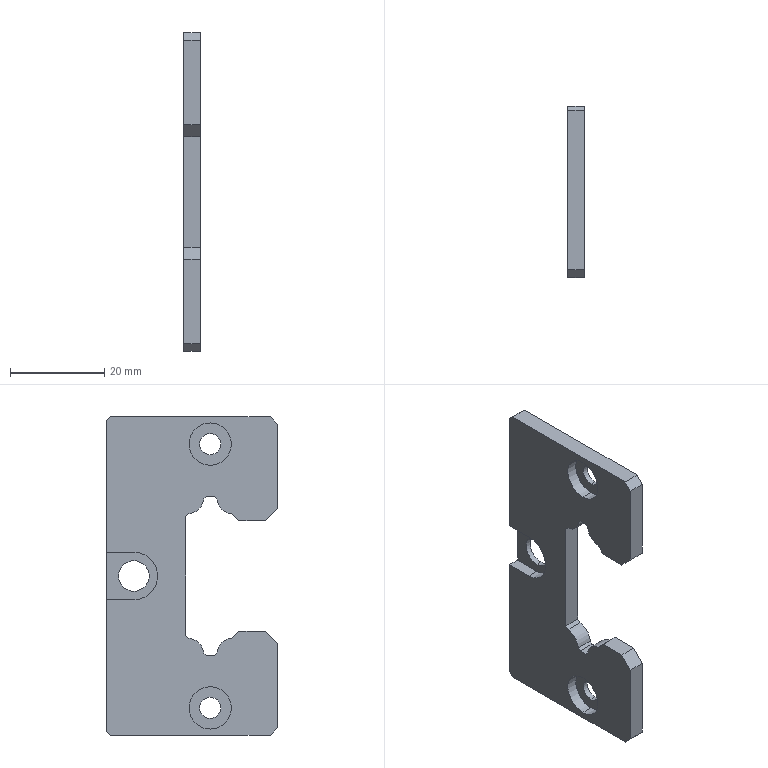Part | STEP file | _MSA35ES | 1 solid | 46 faces | box 3.6 x 36.3 x 67.6 mm | volume 6318 mm3 | plane 31 | cylinder 15 | commonest cylinder face diameters 4.5 x4 7 x4 9 x4 6.5 x2 10.1 x1
STEP:
#1=CARTESIAN_POINT('',(2.4,23.85,30.25));
#2=VERTEX_POINT('',#1);
#3=CARTESIAN_POINT('',(2.4,23.85,25.75));
#4=VERTEX_POINT('',#3);
#5=CARTESIAN_POINT('',(2.4,23.85,28.));
#6=DIRECTION('',(1.,0.,0.));
#7=DIRECTION('',(0.,0.,-1.));
#8=AXIS2_PLACEMENT_3D('',#5,#6,#7);
#9=CIRCLE('',#8,2.25);
#10=EDGE_CURVE('',#2,#4,#9,.T.);
#11=ORIENTED_EDGE('',*,*,#10,.F.);
#12=CARTESIAN_POINT('',(3.6,23.85,30.25));
#13=VERTEX_POINT('',#12);
#14=CARTESIAN_POINT('',(3.6,23.85,30.25));
#15=DIRECTION('',(1.,0.,0.));
#16=VECTOR('',#15,1000.);
#17=LINE('',#14,#16);
#18=EDGE_CURVE('',#2,#13,#17,.T.);
#19=ORIENTED_EDGE('',*,*,#18,.T.);
#20=CARTESIAN_POINT('',(3.6,23.85,25.75));
#21=VERTEX_POINT('',#20);
#22=CARTESIAN_POINT('',(3.6,23.85,28.));
#23=DIRECTION('',(-1.,0.,0.));
#24=DIRECTION('',(0.,0.,-1.));
#25=AXIS2_PLACEMENT_3D('',#22,#23,#24);
#26=CIRCLE('',#25,2.25);
#27=EDGE_CURVE('',#21,#13,#26,.T.);
#28=ORIENTED_EDGE('',*,*,#27,.F.);
#29=CARTESIAN_POINT('',(3.6,23.85,25.75));
#30=DIRECTION('',(1.,0.,0.));
#31=VECTOR('',#30,1000.);
#32=LINE('',#29,#31);
#33=EDGE_CURVE('',#4,#21,#32,.T.);
#34=ORIENTED_EDGE('',*,*,#33,.F.);
#35=EDGE_LOOP('',(#11,#19,#28,#34));
#36=FACE_OUTER_BOUND('',#35,.T.);
#37=CARTESIAN_POINT('',(3.6,23.85,28.));
#38=DIRECTION('',(1.,0.,0.));
#39=DIRECTION('',(0.,0.,-1.));
#40=AXIS2_PLACEMENT_3D('',#37,#38,#39);
#41=CYLINDRICAL_SURFACE('',#40,2.25);
#42=ADVANCED_FACE('',(#36),#41,.F.);
#43=CARTESIAN_POINT('',(2.4,40.05,3.25));
#44=VERTEX_POINT('',#43);
#45=CARTESIAN_POINT('',(2.4,40.05,-3.25));
#46=VERTEX_POINT('',#45);
#47=CARTESIAN_POINT('',(2.4,40.05,0.));
#48=DIRECTION('',(1.,0.,0.));
#49=DIRECTION('',(0.,0.,-1.));
#50=AXIS2_PLACEMENT_3D('',#47,#48,#49);
#51=CIRCLE('',#50,3.25);
#52=EDGE_CURVE('',#44,#46,#51,.T.);
#53=ORIENTED_EDGE('',*,*,#52,.F.);
#54=CARTESIAN_POINT('',(3.6,40.05,3.25));
#55=VERTEX_POINT('',#54);
#56=CARTESIAN_POINT('',(3.6,40.05,3.25));
#57=DIRECTION('',(1.,0.,0.));
#58=VECTOR('',#57,1000.);
#59=LINE('',#56,#58);
#60=EDGE_CURVE('',#44,#55,#59,.T.);
#61=ORIENTED_EDGE('',*,*,#60,.T.);
#62=CARTESIAN_POINT('',(3.6,40.05,-3.25));
#63=VERTEX_POINT('',#62);
#64=CARTESIAN_POINT('',(3.6,40.05,0.));
#65=DIRECTION('',(-1.,0.,0.));
#66=DIRECTION('',(0.,0.,-1.));
#67=AXIS2_PLACEMENT_3D('',#64,#65,#66);
#68=CIRCLE('',#67,3.25);
#69=EDGE_CURVE('',#63,#55,#68,.T.);
#70=ORIENTED_EDGE('',*,*,#69,.F.);
#71=CARTESIAN_POINT('',(3.6,40.05,-3.25));
#72=DIRECTION('',(1.,0.,0.));
#73=VECTOR('',#72,1000.);
#74=LINE('',#71,#73);
#75=EDGE_CURVE('',#46,#63,#74,.T.);
#76=ORIENTED_EDGE('',*,*,#75,.F.);
#77=EDGE_LOOP('',(#53,#61,#70,#76));
#78=FACE_OUTER_BOUND('',#77,.T.);
#79=CARTESIAN_POINT('',(3.6,40.05,0.));
#80=DIRECTION('',(1.,0.,0.));
#81=DIRECTION('',(0.,0.,-1.));
#82=AXIS2_PLACEMENT_3D('',#79,#80,#81);
#83=CYLINDRICAL_SURFACE('',#82,3.25);
#84=ADVANCED_FACE('',(#78),#83,.F.);
#85=CARTESIAN_POINT('',(2.4,23.85,-25.75));
#86=VERTEX_POINT('',#85);
#87=CARTESIAN_POINT('',(2.4,23.85,-30.25));
#88=VERTEX_POINT('',#87);
#89=CARTESIAN_POINT('',(2.4,23.85,-28.));
#90=DIRECTION('',(1.,0.,0.));
#91=DIRECTION('',(0.,0.,-1.));
#92=AXIS2_PLACEMENT_3D('',#89,#90,#91);
#93=CIRCLE('',#92,2.25);
#94=EDGE_CURVE('',#86,#88,#93,.T.);
#95=ORIENTED_EDGE('',*,*,#94,.F.);
#96=CARTESIAN_POINT('',(3.6,23.85,-25.75));
#97=VERTEX_POINT('',#96);
#98=CARTESIAN_POINT('',(3.6,23.85,-25.75));
#99=DIRECTION('',(1.,0.,0.));
#100=VECTOR('',#99,1000.);
#101=LINE('',#98,#100);
#102=EDGE_CURVE('',#86,#97,#101,.T.);
#103=ORIENTED_EDGE('',*,*,#102,.T.);
#104=CARTESIAN_POINT('',(3.6,23.85,-30.25));
#105=VERTEX_POINT('',#104);
#106=CARTESIAN_POINT('',(3.6,23.85,-28.));
#107=DIRECTION('',(-1.,0.,0.));
#108=DIRECTION('',(0.,0.,-1.));
#109=AXIS2_PLACEMENT_3D('',#106,#107,#108);
#110=CIRCLE('',#109,2.25);
#111=EDGE_CURVE('',#105,#97,#110,.T.);
#112=ORIENTED_EDGE('',*,*,#111,.F.);
#113=CARTESIAN_POINT('',(3.6,23.85,-30.25));
#114=DIRECTION('',(1.,0.,0.));
#115=VECTOR('',#114,1000.);
#116=LINE('',#113,#115);
#117=EDGE_CURVE('',#88,#105,#116,.T.);
#118=ORIENTED_EDGE('',*,*,#117,.F.);
#119=EDGE_LOOP('',(#95,#103,#112,#118));
#120=FACE_OUTER_BOUND('',#119,.T.);
#121=CARTESIAN_POINT('',(3.6,23.85,-28.));
#122=DIRECTION('',(1.,0.,0.));
#123=DIRECTION('',(0.,0.,-1.));
#124=AXIS2_PLACEMENT_3D('',#121,#122,#123);
#125=CYLINDRICAL_SURFACE('',#124,2.25);
#126=ADVANCED_FACE('',(#120),#125,.F.);
#127=CARTESIAN_POINT('',(0.,23.85,-32.5));
#128=VERTEX_POINT('',#127);
#129=CARTESIAN_POINT('',(0.,23.85,-23.5));
#130=VERTEX_POINT('',#129);
#131=CARTESIAN_POINT('',(0.,23.85,-28.));
#132=DIRECTION('',(-1.,0.,0.));
#133=DIRECTION('',(0.,0.,-1.));
#134=AXIS2_PLACEMENT_3D('',#131,#132,#133);
#135=CIRCLE('',#134,4.5);
#136=EDGE_CURVE('',#128,#130,#135,.T.);
#137=ORIENTED_EDGE('',*,*,#136,.T.);
#138=CARTESIAN_POINT('',(2.4,23.85,-23.5));
#139=VERTEX_POINT('',#138);
#140=CARTESIAN_POINT('',(2.4,23.85,-23.5));
#141=DIRECTION('',(1.,0.,0.));
#142=VECTOR('',#141,1000.);
#143=LINE('',#140,#142);
#144=EDGE_CURVE('',#130,#139,#143,.T.);
#145=ORIENTED_EDGE('',*,*,#144,.T.);
#146=CARTESIAN_POINT('',(2.4,23.85,-32.5));
#147=VERTEX_POINT('',#146);
#148=CARTESIAN_POINT('',(2.4,23.85,-28.));
#149=DIRECTION('',(1.,0.,0.));
#150=DIRECTION('',(0.,0.,-1.));
#151=AXIS2_PLACEMENT_3D('',#148,#149,#150);
#152=CIRCLE('',#151,4.5);
#153=EDGE_CURVE('',#139,#147,#152,.T.);
#154=ORIENTED_EDGE('',*,*,#153,.T.);
#155=CARTESIAN_POINT('',(2.4,23.85,-32.5));
#156=DIRECTION('',(1.,0.,0.));
#157=VECTOR('',#156,1000.);
#158=LINE('',#155,#157);
#159=EDGE_CURVE('',#128,#147,#158,.T.);
#160=ORIENTED_EDGE('',*,*,#159,.F.);
#161=EDGE_LOOP('',(#137,#145,#154,#160));
#162=FACE_OUTER_BOUND('',#161,.T.);
#163=CARTESIAN_POINT('',(2.4,23.85,-28.));
#164=DIRECTION('',(1.,0.,0.));
#165=DIRECTION('',(0.,0.,-1.));
#166=AXIS2_PLACEMENT_3D('',#163,#164,#165);
#167=CYLINDRICAL_SURFACE('',#166,4.5);
#168=ADVANCED_FACE('',(#162),#167,.F.);
#169=CARTESIAN_POINT('',(0.,23.85,23.5));
#170=VERTEX_POINT('',#169);
#171=CARTESIAN_POINT('',(0.,23.85,32.5));
#172=VERTEX_POINT('',#171);
#173=CARTESIAN_POINT('',(0.,23.85,28.));
#174=DIRECTION('',(-1.,0.,0.));
#175=DIRECTION('',(0.,0.,-1.));
#176=AXIS2_PLACEMENT_3D('',#173,#174,#175);
#177=CIRCLE('',#176,4.5);
#178=EDGE_CURVE('',#170,#172,#177,.T.);
#179=ORIENTED_EDGE('',*,*,#178,.T.);
#180=CARTESIAN_POINT('',(2.4,23.85,32.5));
#181=VERTEX_POINT('',#180);
#182=CARTESIAN_POINT('',(2.4,23.85,32.5));
#183=DIRECTION('',(1.,0.,0.));
#184=VECTOR('',#183,1000.);
#185=LINE('',#182,#184);
#186=EDGE_CURVE('',#172,#181,#185,.T.);
#187=ORIENTED_EDGE('',*,*,#186,.T.);
#188=CARTESIAN_POINT('',(2.4,23.85,23.5));
#189=VERTEX_POINT('',#188);
#190=CARTESIAN_POINT('',(2.4,23.85,28.));
#191=DIRECTION('',(1.,0.,0.));
#192=DIRECTION('',(0.,0.,-1.));
#193=AXIS2_PLACEMENT_3D('',#190,#191,#192);
#194=CIRCLE('',#193,4.5);
#195=EDGE_CURVE('',#181,#189,#194,.T.);
#196=ORIENTED_EDGE('',*,*,#195,.T.);
#197=CARTESIAN_POINT('',(2.4,23.85,23.5));
#198=DIRECTION('',(1.,0.,0.));
#199=VECTOR('',#198,1000.);
#200=LINE('',#197,#199);
#201=EDGE_CURVE('',#170,#189,#200,.T.);
#202=ORIENTED_EDGE('',*,*,#201,.F.);
#203=EDGE_LOOP('',(#179,#187,#196,#202));
#204=FACE_OUTER_BOUND('',#203,.T.);
#205=CARTESIAN_POINT('',(2.4,23.85,28.));
#206=DIRECTION('',(1.,0.,0.));
#207=DIRECTION('',(0.,0.,-1.));
#208=AXIS2_PLACEMENT_3D('',#205,#206,#207);
#209=CYLINDRICAL_SURFACE('',#208,4.5);
#210=ADVANCED_FACE('',(#204),#209,.F.);
#211=CARTESIAN_POINT('',(3.6,22.395,-16.354));
#212=VERTEX_POINT('',#211);
#213=CARTESIAN_POINT('',(3.6,19.248,-13.206));
#214=VERTEX_POINT('',#213);
#215=CARTESIAN_POINT('',(3.6,18.912,-16.69));
#216=DIRECTION('',(1.,0.,0.));
#217=DIRECTION('',(0.,0.,-1.));
#218=AXIS2_PLACEMENT_3D('',#215,#216,#217);
#219=CIRCLE('',#218,3.5);
#220=EDGE_CURVE('',#212,#214,#219,.T.);
#221=ORIENTED_EDGE('',*,*,#220,.T.);
#222=CARTESIAN_POINT('',(3.6,17.741,-11.7));
#223=VERTEX_POINT('',#222);
#224=CARTESIAN_POINT('',(3.6,19.248,-13.206));
#225=DIRECTION('',(0.,-0.7071,0.7071));
#226=VECTOR('',#225,1000.);
#227=LINE('',#224,#226);
#228=EDGE_CURVE('',#214,#223,#227,.T.);
#229=ORIENTED_EDGE('',*,*,#228,.T.);
#230=CARTESIAN_POINT('',(3.6,12.159,-11.7));
#231=VERTEX_POINT('',#230);
#232=CARTESIAN_POINT('',(3.6,0.,-11.7));
#233=DIRECTION('',(0.,-1.,0.));
#234=VECTOR('',#233,1000.);
#235=LINE('',#232,#234);
#236=EDGE_CURVE('',#223,#231,#235,.T.);
#237=ORIENTED_EDGE('',*,*,#236,.T.);
#238=CARTESIAN_POINT('',(3.6,9.55,-14.309));
#239=VERTEX_POINT('',#238);
#240=CARTESIAN_POINT('',(3.6,12.159,-11.7));
#241=DIRECTION('',(0.,-0.7071,-0.7071));
#242=VECTOR('',#241,1000.);
#243=LINE('',#240,#242);
#244=EDGE_CURVE('',#231,#239,#243,.T.);
#245=ORIENTED_EDGE('',*,*,#244,.T.);
#246=CARTESIAN_POINT('',(3.6,9.55,-32.22));
#247=VERTEX_POINT('',#246);
#248=CARTESIAN_POINT('',(3.6,9.55,0.));
#249=DIRECTION('',(0.,0.,-1.));
#250=VECTOR('',#249,1000.);
#251=LINE('',#248,#250);
#252=EDGE_CURVE('',#239,#247,#251,.T.);
#253=ORIENTED_EDGE('',*,*,#252,.T.);
#254=CARTESIAN_POINT('',(3.6,11.13,-33.8));
#255=VERTEX_POINT('',#254);
#256=CARTESIAN_POINT('',(3.6,9.55,-32.22));
#257=DIRECTION('',(0.,0.7071,-0.7071));
#258=VECTOR('',#257,1000.);
#259=LINE('',#256,#258);
#260=EDGE_CURVE('',#247,#255,#259,.T.);
#261=ORIENTED_EDGE('',*,*,#260,.T.);
#262=CARTESIAN_POINT('',(3.6,44.97,-33.8));
#263=VERTEX_POINT('',#262);
#264=CARTESIAN_POINT('',(3.6,0.,-33.8));
#265=DIRECTION('',(0.,1.,0.));
#266=VECTOR('',#265,1000.);
#267=LINE('',#264,#266);
#268=EDGE_CURVE('',#255,#263,#267,.T.);
#269=ORIENTED_EDGE('',*,*,#268,.T.);
#270=CARTESIAN_POINT('',(3.6,45.85,-32.92));
#271=VERTEX_POINT('',#270);
#272=CARTESIAN_POINT('',(3.6,44.97,-33.8));
#273=DIRECTION('',(0.,0.7071,0.7071));
#274=VECTOR('',#273,1000.);
#275=LINE('',#272,#274);
#276=EDGE_CURVE('',#263,#271,#275,.T.);
#277=ORIENTED_EDGE('',*,*,#276,.T.);
#278=CARTESIAN_POINT('',(3.6,45.85,32.92));
#279=VERTEX_POINT('',#278);
#280=CARTESIAN_POINT('',(3.6,45.85,0.));
#281=DIRECTION('',(0.,0.,1.));
#282=VECTOR('',#281,1000.);
#283=LINE('',#280,#282);
#284=EDGE_CURVE('',#271,#279,#283,.T.);
#285=ORIENTED_EDGE('',*,*,#284,.T.);
#286=CARTESIAN_POINT('',(3.6,44.97,33.8));
#287=VERTEX_POINT('',#286);
#288=CARTESIAN_POINT('',(3.6,45.85,32.92));
#289=DIRECTION('',(0.,-0.7071,0.7071));
#290=VECTOR('',#289,1000.);
#291=LINE('',#288,#290);
#292=EDGE_CURVE('',#279,#287,#291,.T.);
#293=ORIENTED_EDGE('',*,*,#292,.T.);
#294=CARTESIAN_POINT('',(3.6,11.13,33.8));
#295=VERTEX_POINT('',#294);
#296=CARTESIAN_POINT('',(3.6,0.,33.8));
#297=DIRECTION('',(0.,-1.,0.));
#298=VECTOR('',#297,1000.);
#299=LINE('',#296,#298);
#300=EDGE_CURVE('',#287,#295,#299,.T.);
#301=ORIENTED_EDGE('',*,*,#300,.T.);
#302=CARTESIAN_POINT('',(3.6,9.55,32.22));
#303=VERTEX_POINT('',#302);
#304=CARTESIAN_POINT('',(3.6,11.13,33.8));
#305=DIRECTION('',(0.,-0.7071,-0.7071));
#306=VECTOR('',#305,1000.);
#307=LINE('',#304,#306);
#308=EDGE_CURVE('',#295,#303,#307,.T.);
#309=ORIENTED_EDGE('',*,*,#308,.T.);
#310=CARTESIAN_POINT('',(3.6,9.55,14.308));
#311=VERTEX_POINT('',#310);
#312=CARTESIAN_POINT('',(3.6,9.55,0.));
#313=DIRECTION('',(0.,0.,-1.));
#314=VECTOR('',#313,1000.);
#315=LINE('',#312,#314);
#316=EDGE_CURVE('',#303,#311,#315,.T.);
#317=ORIENTED_EDGE('',*,*,#316,.T.);
#318=CARTESIAN_POINT('',(3.6,12.159,11.7));
#319=VERTEX_POINT('',#318);
#320=CARTESIAN_POINT('',(3.6,9.55,14.309));
#321=DIRECTION('',(0.,0.7071,-0.7071));
#322=VECTOR('',#321,1000.);
#323=LINE('',#320,#322);
#324=EDGE_CURVE('',#311,#319,#323,.T.);
#325=ORIENTED_EDGE('',*,*,#324,.T.);
#326=CARTESIAN_POINT('',(3.6,17.741,11.7));
#327=VERTEX_POINT('',#326);
#328=CARTESIAN_POINT('',(3.6,0.,11.7));
#329=DIRECTION('',(0.,1.,0.));
#330=VECTOR('',#329,1000.);
#331=LINE('',#328,#330);
#332=EDGE_CURVE('',#319,#327,#331,.T.);
#333=ORIENTED_EDGE('',*,*,#332,.T.);
#334=CARTESIAN_POINT('',(3.6,19.248,13.206));
#335=VERTEX_POINT('',#334);
#336=CARTESIAN_POINT('',(3.6,17.741,11.7));
#337=DIRECTION('',(0.,0.7071,0.7071));
#338=VECTOR('',#337,1000.);
#339=LINE('',#336,#338);
#340=EDGE_CURVE('',#327,#335,#339,.T.);
#341=ORIENTED_EDGE('',*,*,#340,.T.);
#342=CARTESIAN_POINT('',(3.6,22.395,16.354));
#343=VERTEX_POINT('',#342);
#344=CARTESIAN_POINT('',(3.6,18.912,16.69));
#345=DIRECTION('',(1.,0.,0.));
#346=DIRECTION('',(0.,0.,-1.));
#347=AXIS2_PLACEMENT_3D('',#344,#345,#346);
#348=CIRCLE('',#347,3.5);
#349=EDGE_CURVE('',#335,#343,#348,.T.);
#350=ORIENTED_EDGE('',*,*,#349,.T.);
#351=CARTESIAN_POINT('',(3.6,22.941,16.9));
#352=VERTEX_POINT('',#351);
#353=CARTESIAN_POINT('',(3.6,22.941,16.9));
#354=DIRECTION('',(0.,-0.7071,-0.7071));
#355=VECTOR('',#354,1000.);
#356=LINE('',#353,#355);
#357=EDGE_CURVE('',#352,#343,#356,.T.);
#358=ORIENTED_EDGE('',*,*,#357,.F.);
#359=CARTESIAN_POINT('',(3.6,24.659,16.9));
#360=VERTEX_POINT('',#359);
#361=CARTESIAN_POINT('',(3.6,24.659,16.9));
#362=DIRECTION('',(0.,-1.,0.));
#363=VECTOR('',#362,1000.);
#364=LINE('',#361,#363);
#365=EDGE_CURVE('',#360,#352,#364,.T.);
#366=ORIENTED_EDGE('',*,*,#365,.F.);
#367=CARTESIAN_POINT('',(3.6,25.206,16.352));
#368=VERTEX_POINT('',#367);
#369=CARTESIAN_POINT('',(3.6,25.206,16.352));
#370=DIRECTION('',(0.,-0.7071,0.7071));
#371=VECTOR('',#370,1000.);
#372=LINE('',#369,#371);
#373=EDGE_CURVE('',#368,#360,#372,.T.);
#374=ORIENTED_EDGE('',*,*,#373,.F.);
#375=CARTESIAN_POINT('',(3.6,28.352,13.206));
#376=VERTEX_POINT('',#375);
#377=CARTESIAN_POINT('',(3.6,28.69,16.69));
#378=DIRECTION('',(1.,0.,0.));
#379=DIRECTION('',(0.,0.,-1.));
#380=AXIS2_PLACEMENT_3D('',#377,#378,#379);
#381=CIRCLE('',#380,3.5);
#382=EDGE_CURVE('',#368,#376,#381,.T.);
#383=ORIENTED_EDGE('',*,*,#382,.T.);
#384=CARTESIAN_POINT('',(3.6,29.,12.559));
#385=VERTEX_POINT('',#384);
#386=CARTESIAN_POINT('',(3.6,29.,12.559));
#387=DIRECTION('',(0.,-0.7071,0.7071));
#388=VECTOR('',#387,1000.);
#389=LINE('',#386,#388);
#390=EDGE_CURVE('',#385,#376,#389,.T.);
#391=ORIENTED_EDGE('',*,*,#390,.F.);
#392=CARTESIAN_POINT('',(3.6,29.,-12.559));
#393=VERTEX_POINT('',#392);
#394=CARTESIAN_POINT('',(3.6,29.,0.));
#395=DIRECTION('',(0.,0.,-1.));
#396=VECTOR('',#395,1000.);
#397=LINE('',#394,#396);
#398=EDGE_CURVE('',#385,#393,#397,.T.);
#399=ORIENTED_EDGE('',*,*,#398,.T.);
#400=CARTESIAN_POINT('',(3.6,28.352,-13.206));
#401=VERTEX_POINT('',#400);
#402=CARTESIAN_POINT('',(3.6,28.352,-13.206));
#403=DIRECTION('',(0.,0.7071,0.7071));
#404=VECTOR('',#403,1000.);
#405=LINE('',#402,#404);
#406=EDGE_CURVE('',#401,#393,#405,.T.);
#407=ORIENTED_EDGE('',*,*,#406,.F.);
#408=CARTESIAN_POINT('',(3.6,25.206,-16.352));
#409=VERTEX_POINT('',#408);
#410=CARTESIAN_POINT('',(3.6,28.69,-16.69));
#411=DIRECTION('',(1.,0.,0.));
#412=DIRECTION('',(0.,0.,-1.));
#413=AXIS2_PLACEMENT_3D('',#410,#411,#412);
#414=CIRCLE('',#413,3.5);
#415=EDGE_CURVE('',#401,#409,#414,.T.);
#416=ORIENTED_EDGE('',*,*,#415,.T.);
#417=CARTESIAN_POINT('',(3.6,24.659,-16.9));
#418=VERTEX_POINT('',#417);
#419=CARTESIAN_POINT('',(3.6,24.659,-16.9));
#420=DIRECTION('',(0.,0.7071,0.7071));
#421=VECTOR('',#420,1000.);
#422=LINE('',#419,#421);
#423=EDGE_CURVE('',#418,#409,#422,.T.);
#424=ORIENTED_EDGE('',*,*,#423,.F.);
#425=CARTESIAN_POINT('',(3.6,22.941,-16.9));
#426=VERTEX_POINT('',#425);
#427=CARTESIAN_POINT('',(3.6,22.941,-16.9));
#428=DIRECTION('',(0.,1.,0.));
#429=VECTOR('',#428,1000.);
#430=LINE('',#427,#429);
#431=EDGE_CURVE('',#426,#418,#430,.T.);
#432=ORIENTED_EDGE('',*,*,#431,.F.);
#433=CARTESIAN_POINT('',(3.6,22.395,-16.354));
#434=DIRECTION('',(0.,0.7071,-0.7071));
#435=VECTOR('',#434,1000.);
#436=LINE('',#433,#435);
#437=EDGE_CURVE('',#212,#426,#436,.T.);
#438=ORIENTED_EDGE('',*,*,#437,.F.);
#439=EDGE_LOOP('',(#221,#229,#237,#245,#253,#261,#269,#277,#285,#293,#301,#309,#317,#325,#333,#341,#350,#358,#366,#374,#383,#391,#399,#407,#416,#424,#432,#438));
#440=FACE_OUTER_BOUND('',#439,.T.);
#441=ORIENTED_EDGE('',*,*,#27,.T.);
#442=CARTESIAN_POINT('',(3.6,23.85,28.));
#443=DIRECTION('',(-1.,0.,0.));
#444=DIRECTION('',(0.,0.,-1.));
#445=AXIS2_PLACEMENT_3D('',#442,#443,#444);
#446=CIRCLE('',#445,2.25);
#447=EDGE_CURVE('',#13,#21,#446,.T.);
#448=ORIENTED_EDGE('',*,*,#447,.T.);
#449=EDGE_LOOP('',(#441,#448));
#450=FACE_BOUND('',#449,.T.);
#451=ORIENTED_EDGE('',*,*,#69,.T.);
#452=CARTESIAN_POINT('',(3.6,40.05,0.));
#453=DIRECTION('',(-1.,0.,0.));
#454=DIRECTION('',(0.,0.,-1.));
#455=AXIS2_PLACEMENT_3D('',#452,#453,#454);
#456=CIRCLE('',#455,3.25);
#457=EDGE_CURVE('',#55,#63,#456,.T.);
#458=ORIENTED_EDGE('',*,*,#457,.T.);
#459=EDGE_LOOP('',(#451,#458));
#460=FACE_BOUND('',#459,.T.);
#461=ORIENTED_EDGE('',*,*,#111,.T.);
#462=CARTESIAN_POINT('',(3.6,23.85,-28.));
#463=DIRECTION('',(-1.,0.,0.));
#464=DIRECTION('',(0.,0.,-1.));
#465=AXIS2_PLACEMENT_3D('',#462,#463,#464);
#466=CIRCLE('',#465,2.25);
#467=EDGE_CURVE('',#97,#105,#466,.T.);
#468=ORIENTED_EDGE('',*,*,#467,.T.);
#469=EDGE_LOOP('',(#461,#468));
#470=FACE_BOUND('',#469,.T.);
#471=CARTESIAN_POINT('',(3.6,0.,0.));
#472=DIRECTION('',(1.,0.,0.));
#473=DIRECTION('',(0.,0.,-1.));
#474=AXIS2_PLACEMENT_3D('',#471,#472,#473);
#475=PLANE('',#474);
#476=ADVANCED_FACE('',(#440,#450,#460,#470),#475,.T.);
#477=CARTESIAN_POINT('',(0.,17.741,-11.7));
#478=VERTEX_POINT('',#477);
#479=CARTESIAN_POINT('',(3.75,17.741,-11.7));
#480=DIRECTION('',(1.,0.,0.));
#481=VECTOR('',#480,1000.);
#482=LINE('',#479,#481);
#483=EDGE_CURVE('',#478,#223,#482,.T.);
#484=ORIENTED_EDGE('',*,*,#483,.T.);
#485=ORIENTED_EDGE('',*,*,#228,.F.);
#486=CARTESIAN_POINT('',(0.,19.248,-13.206));
#487=VERTEX_POINT('',#486);
#488=CARTESIAN_POINT('',(3.75,19.248,-13.206));
#489=DIRECTION('',(-1.,0.,0.));
#490=VECTOR('',#489,1000.);
#491=LINE('',#488,#490);
#492=EDGE_CURVE('',#214,#487,#491,.T.);
#493=ORIENTED_EDGE('',*,*,#492,.T.);
#494=CARTESIAN_POINT('',(0.,17.741,-11.7));
#495=DIRECTION('',(0.,-0.7071,0.7071));
#496=VECTOR('',#495,1000.);
#497=LINE('',#494,#496);
#498=EDGE_CURVE('',#487,#478,#497,.T.);
#499=ORIENTED_EDGE('',*,*,#498,.T.);
#500=EDGE_LOOP('',(#484,#485,#493,#499));
#501=FACE_OUTER_BOUND('',#500,.T.);
#502=CARTESIAN_POINT('',(3.75,17.741,-11.7));
#503=DIRECTION('',(0.,0.7071,0.7071));
#504=DIRECTION('',(0.,-0.7071,0.7071));
#505=AXIS2_PLACEMENT_3D('',#502,#503,#504);
#506=PLANE('',#505);
#507=ADVANCED_FACE('',(#501),#506,.T.);
#508=CARTESIAN_POINT('',(0.,22.395,-16.354));
#509=VERTEX_POINT('',#508);
#510=CARTESIAN_POINT('',(0.,18.912,-16.69));
#511=DIRECTION('',(1.,0.,0.));
#512=DIRECTION('',(0.,0.,-1.));
#513=AXIS2_PLACEMENT_3D('',#510,#511,#512);
#514=CIRCLE('',#513,3.5);
#515=EDGE_CURVE('',#509,#487,#514,.T.);
#516=ORIENTED_EDGE('',*,*,#515,.T.);
#517=ORIENTED_EDGE('',*,*,#492,.F.);
#518=ORIENTED_EDGE('',*,*,#220,.F.);
#519=CARTESIAN_POINT('',(3.75,22.395,-16.354));
#520=DIRECTION('',(-1.,0.,0.));
#521=VECTOR('',#520,1000.);
#522=LINE('',#519,#521);
#523=EDGE_CURVE('',#212,#509,#522,.T.);
#524=ORIENTED_EDGE('',*,*,#523,.T.);
#525=EDGE_LOOP('',(#516,#517,#518,#524));
#526=FACE_OUTER_BOUND('',#525,.T.);
#527=CARTESIAN_POINT('',(3.75,18.912,-16.69));
#528=DIRECTION('',(1.,0.,0.));
#529=DIRECTION('',(0.,0.,-1.));
#530=AXIS2_PLACEMENT_3D('',#527,#528,#529);
#531=CYLINDRICAL_SURFACE('',#530,3.5);
#532=ADVANCED_FACE('',(#526),#531,.T.);
#533=CARTESIAN_POINT('',(0.,28.352,-13.206));
#534=VERTEX_POINT('',#533);
#535=CARTESIAN_POINT('',(0.,25.206,-16.352));
#536=VERTEX_POINT('',#535);
#537=CARTESIAN_POINT('',(0.,28.69,-16.69));
#538=DIRECTION('',(1.,0.,0.));
#539=DIRECTION('',(0.,0.,-1.));
#540=AXIS2_PLACEMENT_3D('',#537,#538,#539);
#541=CIRCLE('',#540,3.5);
#542=EDGE_CURVE('',#534,#536,#541,.T.);
#543=ORIENTED_EDGE('',*,*,#542,.T.);
#544=CARTESIAN_POINT('',(3.75,25.206,-16.352));
#545=DIRECTION('',(1.,0.,0.));
#546=VECTOR('',#545,1000.);
#547=LINE('',#544,#546);
#548=EDGE_CURVE('',#536,#409,#547,.T.);
#549=ORIENTED_EDGE('',*,*,#548,.T.);
#550=ORIENTED_EDGE('',*,*,#415,.F.);
#551=CARTESIAN_POINT('',(3.75,28.352,-13.206));
#552=DIRECTION('',(-1.,0.,0.));
#553=VECTOR('',#552,1000.);
#554=LINE('',#551,#553);
#555=EDGE_CURVE('',#401,#534,#554,.T.);
#556=ORIENTED_EDGE('',*,*,#555,.T.);
#557=EDGE_LOOP('',(#543,#549,#550,#556));
#558=FACE_OUTER_BOUND('',#557,.T.);
#559=CARTESIAN_POINT('',(3.75,28.69,-16.69));
#560=DIRECTION('',(1.,0.,0.));
#561=DIRECTION('',(0.,0.,-1.));
#562=AXIS2_PLACEMENT_3D('',#559,#560,#561);
#563=CYLINDRICAL_SURFACE('',#562,3.5);
#564=ADVANCED_FACE('',(#558),#563,.T.);
#565=CARTESIAN_POINT('',(0.,29.,-12.559));
#566=VERTEX_POINT('',#565);
#567=CARTESIAN_POINT('',(3.75,29.,-12.559));
#568=DIRECTION('',(1.,0.,0.));
#569=VECTOR('',#568,1000.);
#570=LINE('',#567,#569);
#571=EDGE_CURVE('',#566,#393,#570,.T.);
#572=ORIENTED_EDGE('',*,*,#571,.T.);
#573=ORIENTED_EDGE('',*,*,#398,.F.);
#574=CARTESIAN_POINT('',(0.,29.,12.559));
#575=VERTEX_POINT('',#574);
#576=CARTESIAN_POINT('',(3.75,29.,12.559));
#577=DIRECTION('',(-1.,0.,0.));
#578=VECTOR('',#577,1000.);
#579=LINE('',#576,#578);
#580=EDGE_CURVE('',#385,#575,#579,.T.);
#581=ORIENTED_EDGE('',*,*,#580,.T.);
#582=CARTESIAN_POINT('',(0.,29.,-12.559));
#583=DIRECTION('',(0.,0.,-1.));
#584=VECTOR('',#583,1000.);
#585=LINE('',#582,#584);
#586=EDGE_CURVE('',#575,#566,#585,.T.);
#587=ORIENTED_EDGE('',*,*,#586,.T.);
#588=EDGE_LOOP('',(#572,#573,#581,#587));
#589=FACE_OUTER_BOUND('',#588,.T.);
#590=CARTESIAN_POINT('',(3.75,29.,-12.559));
#591=DIRECTION('',(0.,-1.,0.));
#592=DIRECTION('',(0.,0.,-1.));
#593=AXIS2_PLACEMENT_3D('',#590,#591,#592);
#594=PLANE('',#593);
#595=ADVANCED_FACE('',(#589),#594,.T.);
#596=CARTESIAN_POINT('',(0.,25.206,16.352));
#597=VERTEX_POINT('',#596);
#598=CARTESIAN_POINT('',(0.,28.352,13.206));
#599=VERTEX_POINT('',#598);
#600=CARTESIAN_POINT('',(0.,28.69,16.69));
#601=DIRECTION('',(1.,0.,0.));
#602=DIRECTION('',(0.,0.,-1.));
#603=AXIS2_PLACEMENT_3D('',#600,#601,#602);
#604=CIRCLE('',#603,3.5);
#605=EDGE_CURVE('',#597,#599,#604,.T.);
#606=ORIENTED_EDGE('',*,*,#605,.T.);
#607=CARTESIAN_POINT('',(3.75,28.352,13.206));
#608=DIRECTION('',(1.,0.,0.));
#609=VECTOR('',#608,1000.);
#610=LINE('',#607,#609);
#611=EDGE_CURVE('',#599,#376,#610,.T.);
#612=ORIENTED_EDGE('',*,*,#611,.T.);
#613=ORIENTED_EDGE('',*,*,#382,.F.);
#614=CARTESIAN_POINT('',(3.75,25.206,16.352));
#615=DIRECTION('',(-1.,0.,0.));
#616=VECTOR('',#615,1000.);
#617=LINE('',#614,#616);
#618=EDGE_CURVE('',#368,#597,#617,.T.);
#619=ORIENTED_EDGE('',*,*,#618,.T.);
#620=EDGE_LOOP('',(#606,#612,#613,#619));
#621=FACE_OUTER_BOUND('',#620,.T.);
#622=CARTESIAN_POINT('',(3.75,28.69,16.69));
#623=DIRECTION('',(1.,0.,0.));
#624=DIRECTION('',(0.,0.,-1.));
#625=AXIS2_PLACEMENT_3D('',#622,#623,#624);
#626=CYLINDRICAL_SURFACE('',#625,3.5);
#627=ADVANCED_FACE('',(#621),#626,.T.);
#628=CARTESIAN_POINT('',(0.,19.248,13.206));
#629=VERTEX_POINT('',#628);
#630=CARTESIAN_POINT('',(0.,22.395,16.354));
#631=VERTEX_POINT('',#630);
#632=CARTESIAN_POINT('',(0.,18.912,16.69));
#633=DIRECTION('',(1.,0.,0.));
#634=DIRECTION('',(0.,0.,-1.));
#635=AXIS2_PLACEMENT_3D('',#632,#633,#634);
#636=CIRCLE('',#635,3.5);
#637=EDGE_CURVE('',#629,#631,#636,.T.);
#638=ORIENTED_EDGE('',*,*,#637,.T.);
#639=CARTESIAN_POINT('',(3.75,22.395,16.354));
#640=DIRECTION('',(1.,0.,0.));
#641=VECTOR('',#640,1000.);
#642=LINE('',#639,#641);
#643=EDGE_CURVE('',#631,#343,#642,.T.);
#644=ORIENTED_EDGE('',*,*,#643,.T.);
#645=ORIENTED_EDGE('',*,*,#349,.F.);
#646=CARTESIAN_POINT('',(3.75,19.248,13.206));
#647=DIRECTION('',(-1.,0.,0.));
#648=VECTOR('',#647,1000.);
#649=LINE('',#646,#648);
#650=EDGE_CURVE('',#335,#629,#649,.T.);
#651=ORIENTED_EDGE('',*,*,#650,.T.);
#652=EDGE_LOOP('',(#638,#644,#645,#651));
#653=FACE_OUTER_BOUND('',#652,.T.);
#654=CARTESIAN_POINT('',(3.75,18.912,16.69));
#655=DIRECTION('',(1.,0.,0.));
#656=DIRECTION('',(0.,0.,-1.));
#657=AXIS2_PLACEMENT_3D('',#654,#655,#656);
#658=CYLINDRICAL_SURFACE('',#657,3.5);
#659=ADVANCED_FACE('',(#653),#658,.T.);
#660=ORIENTED_EDGE('',*,*,#650,.F.);
#661=ORIENTED_EDGE('',*,*,#340,.F.);
#662=CARTESIAN_POINT('',(0.,17.741,11.7));
#663=VERTEX_POINT('',#662);
#664=CARTESIAN_POINT('',(3.75,17.741,11.7));
#665=DIRECTION('',(-1.,0.,0.));
#666=VECTOR('',#665,1000.);
#667=LINE('',#664,#666);
#668=EDGE_CURVE('',#327,#663,#667,.T.);
#669=ORIENTED_EDGE('',*,*,#668,.T.);
#670=CARTESIAN_POINT('',(0.,19.248,13.206));
#671=DIRECTION('',(0.,0.7071,0.7071));
#672=VECTOR('',#671,1000.);
#673=LINE('',#670,#672);
#674=EDGE_CURVE('',#663,#629,#673,.T.);
#675=ORIENTED_EDGE('',*,*,#674,.T.);
#676=EDGE_LOOP('',(#660,#661,#669,#675));
#677=FACE_OUTER_BOUND('',#676,.T.);
#678=CARTESIAN_POINT('',(3.75,19.248,13.206));
#679=DIRECTION('',(0.,0.7071,-0.7071));
#680=DIRECTION('',(0.,0.7071,0.7071));
#681=AXIS2_PLACEMENT_3D('',#678,#679,#680);
#682=PLANE('',#681);
#683=ADVANCED_FACE('',(#677),#682,.T.);
#684=ORIENTED_EDGE('',*,*,#668,.F.);
#685=ORIENTED_EDGE('',*,*,#332,.F.);
#686=CARTESIAN_POINT('',(0.,12.159,11.7));
#687=VERTEX_POINT('',#686);
#688=CARTESIAN_POINT('',(3.75,12.159,11.7));
#689=DIRECTION('',(-1.,0.,0.));
#690=VECTOR('',#689,1000.);
#691=LINE('',#688,#690);
#692=EDGE_CURVE('',#319,#687,#691,.T.);
#693=ORIENTED_EDGE('',*,*,#692,.T.);
#694=CARTESIAN_POINT('',(0.,17.741,11.7));
#695=DIRECTION('',(0.,1.,0.));
#696=VECTOR('',#695,1000.);
#697=LINE('',#694,#696);
#698=EDGE_CURVE('',#687,#663,#697,.T.);
#699=ORIENTED_EDGE('',*,*,#698,.T.);
#700=EDGE_LOOP('',(#684,#685,#693,#699));
#701=FACE_OUTER_BOUND('',#700,.T.);
#702=CARTESIAN_POINT('',(3.75,17.741,11.7));
#703=DIRECTION('',(0.,0.,-1.));
#704=DIRECTION('',(-1.,0.,0.));
#705=AXIS2_PLACEMENT_3D('',#702,#703,#704);
#706=PLANE('',#705);
#707=ADVANCED_FACE('',(#701),#706,.T.);
#708=ORIENTED_EDGE('',*,*,#692,.F.);
#709=ORIENTED_EDGE('',*,*,#324,.F.);
#710=CARTESIAN_POINT('',(0.,9.55,14.309));
#711=VERTEX_POINT('',#710);
#712=CARTESIAN_POINT('',(3.75,9.55,14.308));
#713=DIRECTION('',(-1.,0.,0.));
#714=VECTOR('',#713,1000.);
#715=LINE('',#712,#714);
#716=EDGE_CURVE('',#311,#711,#715,.T.);
#717=ORIENTED_EDGE('',*,*,#716,.T.);
#718=CARTESIAN_POINT('',(0.,12.159,11.7));
#719=DIRECTION('',(0.,0.7071,-0.7071));
#720=VECTOR('',#719,1000.);
#721=LINE('',#718,#720);
#722=EDGE_CURVE('',#711,#687,#721,.T.);
#723=ORIENTED_EDGE('',*,*,#722,.T.);
#724=EDGE_LOOP('',(#708,#709,#717,#723));
#725=FACE_OUTER_BOUND('',#724,.T.);
#726=CARTESIAN_POINT('',(3.75,12.159,11.7));
#727=DIRECTION('',(0.,-0.7071,-0.7071));
#728=DIRECTION('',(0.,0.7071,-0.7071));
#729=AXIS2_PLACEMENT_3D('',#726,#727,#728);
#730=PLANE('',#729);
#731=ADVANCED_FACE('',(#725),#730,.T.);
#732=ORIENTED_EDGE('',*,*,#316,.F.);
#733=CARTESIAN_POINT('',(0.,9.55,32.22));
#734=VERTEX_POINT('',#733);
#735=CARTESIAN_POINT('',(3.6,9.55,32.22));
#736=DIRECTION('',(1.,0.,0.));
#737=VECTOR('',#736,1000.);
#738=LINE('',#735,#737);
#739=EDGE_CURVE('',#734,#303,#738,.T.);
#740=ORIENTED_EDGE('',*,*,#739,.F.);
#741=CARTESIAN_POINT('',(0.,9.55,32.22));
#742=DIRECTION('',(0.,0.,1.));
#743=VECTOR('',#742,1000.);
#744=LINE('',#741,#743);
#745=EDGE_CURVE('',#711,#734,#744,.T.);
#746=ORIENTED_EDGE('',*,*,#745,.F.);
#747=ORIENTED_EDGE('',*,*,#716,.F.);
#748=EDGE_LOOP('',(#732,#740,#746,#747));
#749=FACE_OUTER_BOUND('',#748,.T.);
#750=CARTESIAN_POINT('',(3.6,9.55,32.22));
#751=DIRECTION('',(0.,1.,0.));
#752=DIRECTION('',(0.,0.,1.));
#753=AXIS2_PLACEMENT_3D('',#750,#751,#752);
#754=PLANE('',#753);
#755=ADVANCED_FACE('',(#749),#754,.F.);
#756=ORIENTED_EDGE('',*,*,#739,.T.);
#757=ORIENTED_EDGE('',*,*,#308,.F.);
#758=CARTESIAN_POINT('',(0.,11.13,33.8));
#759=VERTEX_POINT('',#758);
#760=CARTESIAN_POINT('',(3.6,11.13,33.8));
#761=DIRECTION('',(1.,0.,0.));
#762=VECTOR('',#761,1000.);
#763=LINE('',#760,#762);
#764=EDGE_CURVE('',#759,#295,#763,.T.);
#765=ORIENTED_EDGE('',*,*,#764,.F.);
#766=CARTESIAN_POINT('',(0.,11.13,33.8));
#767=DIRECTION('',(0.,0.7071,0.7071));
#768=VECTOR('',#767,1000.);
#769=LINE('',#766,#768);
#770=EDGE_CURVE('',#734,#759,#769,.T.);
#771=ORIENTED_EDGE('',*,*,#770,.F.);
#772=EDGE_LOOP('',(#756,#757,#765,#771));
#773=FACE_OUTER_BOUND('',#772,.T.);
#774=CARTESIAN_POINT('',(3.6,11.13,33.8));
#775=DIRECTION('',(0.,0.7071,-0.7071));
#776=DIRECTION('',(0.,0.7071,0.7071));
#777=AXIS2_PLACEMENT_3D('',#774,#775,#776);
#778=PLANE('',#777);
#779=ADVANCED_FACE('',(#773),#778,.F.);
#780=ORIENTED_EDGE('',*,*,#764,.T.);
#781=ORIENTED_EDGE('',*,*,#300,.F.);
#782=CARTESIAN_POINT('',(0.,44.97,33.8));
#783=VERTEX_POINT('',#782);
#784=CARTESIAN_POINT('',(3.6,44.97,33.8));
#785=DIRECTION('',(1.,0.,0.));
#786=VECTOR('',#785,1000.);
#787=LINE('',#784,#786);
#788=EDGE_CURVE('',#783,#287,#787,.T.);
#789=ORIENTED_EDGE('',*,*,#788,.F.);
#790=CARTESIAN_POINT('',(0.,44.97,33.8));
#791=DIRECTION('',(0.,1.,0.));
#792=VECTOR('',#791,1000.);
#793=LINE('',#790,#792);
#794=EDGE_CURVE('',#759,#783,#793,.T.);
#795=ORIENTED_EDGE('',*,*,#794,.F.);
#796=EDGE_LOOP('',(#780,#781,#789,#795));
#797=FACE_OUTER_BOUND('',#796,.T.);
#798=CARTESIAN_POINT('',(3.6,44.97,33.8));
#799=DIRECTION('',(0.,0.,-1.));
#800=DIRECTION('',(-1.,0.,0.));
#801=AXIS2_PLACEMENT_3D('',#798,#799,#800);
#802=PLANE('',#801);
#803=ADVANCED_FACE('',(#797),#802,.F.);
#804=CARTESIAN_POINT('',(0.,45.85,32.92));
#805=VERTEX_POINT('',#804);
#806=CARTESIAN_POINT('',(0.,45.85,5.05));
#807=VERTEX_POINT('',#806);
#808=CARTESIAN_POINT('',(0.,45.85,-32.92));
#809=DIRECTION('',(0.,0.,-1.));
#810=VECTOR('',#809,1000.);
#811=LINE('',#808,#810);
#812=EDGE_CURVE('',#805,#807,#811,.T.);
#813=ORIENTED_EDGE('',*,*,#812,.F.);
#814=CARTESIAN_POINT('',(3.6,45.85,32.92));
#815=DIRECTION('',(-1.,0.,0.));
#816=VECTOR('',#815,1000.);
#817=LINE('',#814,#816);
#818=EDGE_CURVE('',#279,#805,#817,.T.);
#819=ORIENTED_EDGE('',*,*,#818,.F.);
#820=ORIENTED_EDGE('',*,*,#284,.F.);
#821=CARTESIAN_POINT('',(0.,45.85,-32.92));
#822=VERTEX_POINT('',#821);
#823=CARTESIAN_POINT('',(3.6,45.85,-32.92));
#824=DIRECTION('',(1.,0.,0.));
#825=VECTOR('',#824,1000.);
#826=LINE('',#823,#825);
#827=EDGE_CURVE('',#822,#271,#826,.T.);
#828=ORIENTED_EDGE('',*,*,#827,.F.);
#829=CARTESIAN_POINT('',(0.,45.85,-5.05));
#830=VERTEX_POINT('',#829);
#831=CARTESIAN_POINT('',(0.,45.85,-32.92));
#832=DIRECTION('',(0.,0.,-1.));
#833=VECTOR('',#832,1000.);
#834=LINE('',#831,#833);
#835=EDGE_CURVE('',#830,#822,#834,.T.);
#836=ORIENTED_EDGE('',*,*,#835,.F.);
#837=CARTESIAN_POINT('',(2.4,45.85,-5.05));
#838=VERTEX_POINT('',#837);
#839=CARTESIAN_POINT('',(3.6,45.85,-5.05));
#840=DIRECTION('',(-1.,0.,0.));
#841=VECTOR('',#840,1000.);
#842=LINE('',#839,#841);
#843=EDGE_CURVE('',#838,#830,#842,.T.);
#844=ORIENTED_EDGE('',*,*,#843,.F.);
#845=CARTESIAN_POINT('',(2.4,45.85,5.05));
#846=VERTEX_POINT('',#845);
#847=CARTESIAN_POINT('',(2.4,45.85,-32.92));
#848=DIRECTION('',(0.,0.,-1.));
#849=VECTOR('',#848,1000.);
#850=LINE('',#847,#849);
#851=EDGE_CURVE('',#846,#838,#850,.T.);
#852=ORIENTED_EDGE('',*,*,#851,.F.);
#853=CARTESIAN_POINT('',(3.6,45.85,5.05));
#854=DIRECTION('',(1.,0.,0.));
#855=VECTOR('',#854,1000.);
#856=LINE('',#853,#855);
#857=EDGE_CURVE('',#807,#846,#856,.T.);
#858=ORIENTED_EDGE('',*,*,#857,.F.);
#859=EDGE_LOOP('',(#813,#819,#820,#828,#836,#844,#852,#858));
#860=FACE_OUTER_BOUND('',#859,.T.);
#861=CARTESIAN_POINT('',(3.6,45.85,-32.92));
#862=DIRECTION('',(0.,-1.,0.));
#863=DIRECTION('',(0.,0.,-1.));
#864=AXIS2_PLACEMENT_3D('',#861,#862,#863);
#865=PLANE('',#864);
#866=ADVANCED_FACE('',(#860),#865,.F.);
#867=CARTESIAN_POINT('',(0.,44.97,-33.8));
#868=VERTEX_POINT('',#867);
#869=CARTESIAN_POINT('',(3.6,44.97,-33.8));
#870=DIRECTION('',(-1.,0.,0.));
#871=VECTOR('',#870,1000.);
#872=LINE('',#869,#871);
#873=EDGE_CURVE('',#263,#868,#872,.T.);
#874=ORIENTED_EDGE('',*,*,#873,.F.);
#875=ORIENTED_EDGE('',*,*,#268,.F.);
#876=CARTESIAN_POINT('',(0.,11.13,-33.8));
#877=VERTEX_POINT('',#876);
#878=CARTESIAN_POINT('',(3.6,11.13,-33.8));
#879=DIRECTION('',(1.,0.,0.));
#880=VECTOR('',#879,1000.);
#881=LINE('',#878,#880);
#882=EDGE_CURVE('',#877,#255,#881,.T.);
#883=ORIENTED_EDGE('',*,*,#882,.F.);
#884=CARTESIAN_POINT('',(0.,11.13,-33.8));
#885=DIRECTION('',(0.,-1.,0.));
#886=VECTOR('',#885,1000.);
#887=LINE('',#884,#886);
#888=EDGE_CURVE('',#868,#877,#887,.T.);
#889=ORIENTED_EDGE('',*,*,#888,.F.);
#890=EDGE_LOOP('',(#874,#875,#883,#889));
#891=FACE_OUTER_BOUND('',#890,.T.);
#892=CARTESIAN_POINT('',(3.6,11.13,-33.8));
#893=DIRECTION('',(0.,0.,1.));
#894=DIRECTION('',(1.,0.,0.));
#895=AXIS2_PLACEMENT_3D('',#892,#893,#894);
#896=PLANE('',#895);
#897=ADVANCED_FACE('',(#891),#896,.F.);
#898=ORIENTED_EDGE('',*,*,#882,.T.);
#899=ORIENTED_EDGE('',*,*,#260,.F.);
#900=CARTESIAN_POINT('',(0.,9.55,-32.22));
#901=VERTEX_POINT('',#900);
#902=CARTESIAN_POINT('',(3.6,9.55,-32.22));
#903=DIRECTION('',(1.,0.,0.));
#904=VECTOR('',#903,1000.);
#905=LINE('',#902,#904);
#906=EDGE_CURVE('',#901,#247,#905,.T.);
#907=ORIENTED_EDGE('',*,*,#906,.F.);
#908=CARTESIAN_POINT('',(0.,9.55,-32.22));
#909=DIRECTION('',(0.,-0.7071,0.7071));
#910=VECTOR('',#909,1000.);
#911=LINE('',#908,#910);
#912=EDGE_CURVE('',#877,#901,#911,.T.);
#913=ORIENTED_EDGE('',*,*,#912,.F.);
#914=EDGE_LOOP('',(#898,#899,#907,#913));
#915=FACE_OUTER_BOUND('',#914,.T.);
#916=CARTESIAN_POINT('',(3.6,9.55,-32.22));
#917=DIRECTION('',(0.,0.7071,0.7071));
#918=DIRECTION('',(0.,-0.7071,0.7071));
#919=AXIS2_PLACEMENT_3D('',#916,#917,#918);
#920=PLANE('',#919);
#921=ADVANCED_FACE('',(#915),#920,.F.);
#922=CARTESIAN_POINT('',(0.,9.55,-14.308));
#923=VERTEX_POINT('',#922);
#924=CARTESIAN_POINT('',(0.,9.55,32.22));
#925=DIRECTION('',(0.,0.,1.));
#926=VECTOR('',#925,1000.);
#927=LINE('',#924,#926);
#928=EDGE_CURVE('',#901,#923,#927,.T.);
#929=ORIENTED_EDGE('',*,*,#928,.F.);
#930=ORIENTED_EDGE('',*,*,#906,.T.);
#931=ORIENTED_EDGE('',*,*,#252,.F.);
#932=CARTESIAN_POINT('',(3.6,9.55,-14.309));
#933=DIRECTION('',(1.,0.,0.));
#934=VECTOR('',#933,1000.);
#935=LINE('',#932,#934);
#936=EDGE_CURVE('',#923,#239,#935,.T.);
#937=ORIENTED_EDGE('',*,*,#936,.F.);
#938=EDGE_LOOP('',(#929,#930,#931,#937));
#939=FACE_OUTER_BOUND('',#938,.T.);
#940=CARTESIAN_POINT('',(3.6,9.55,32.22));
#941=DIRECTION('',(0.,1.,0.));
#942=DIRECTION('',(0.,0.,1.));
#943=AXIS2_PLACEMENT_3D('',#940,#941,#942);
#944=PLANE('',#943);
#945=ADVANCED_FACE('',(#939),#944,.F.);
#946=CARTESIAN_POINT('',(0.,12.159,-11.7));
#947=VERTEX_POINT('',#946);
#948=CARTESIAN_POINT('',(3.75,12.159,-11.7));
#949=DIRECTION('',(-1.,0.,0.));
#950=VECTOR('',#949,1000.);
#951=LINE('',#948,#950);
#952=EDGE_CURVE('',#231,#947,#951,.T.);
#953=ORIENTED_EDGE('',*,*,#952,.T.);
#954=CARTESIAN_POINT('',(0.,6.859,-17.));
#955=DIRECTION('',(0.,-0.7071,-0.7071));
#956=VECTOR('',#955,1000.);
#957=LINE('',#954,#956);
#958=EDGE_CURVE('',#947,#923,#957,.T.);
#959=ORIENTED_EDGE('',*,*,#958,.T.);
#960=ORIENTED_EDGE('',*,*,#936,.T.);
#961=ORIENTED_EDGE('',*,*,#244,.F.);
#962=EDGE_LOOP('',(#953,#959,#960,#961));
#963=FACE_OUTER_BOUND('',#962,.T.);
#964=CARTESIAN_POINT('',(3.75,6.859,-17.));
#965=DIRECTION('',(0.,-0.7071,0.7071));
#966=DIRECTION('',(0.,-0.7071,-0.7071));
#967=AXIS2_PLACEMENT_3D('',#964,#965,#966);
#968=PLANE('',#967);
#969=ADVANCED_FACE('',(#963),#968,.T.);
#970=ORIENTED_EDGE('',*,*,#952,.F.);
#971=ORIENTED_EDGE('',*,*,#236,.F.);
#972=ORIENTED_EDGE('',*,*,#483,.F.);
#973=CARTESIAN_POINT('',(0.,12.159,-11.7));
#974=DIRECTION('',(0.,-1.,0.));
#975=VECTOR('',#974,1000.);
#976=LINE('',#973,#975);
#977=EDGE_CURVE('',#478,#947,#976,.T.);
#978=ORIENTED_EDGE('',*,*,#977,.T.);
#979=EDGE_LOOP('',(#970,#971,#972,#978));
#980=FACE_OUTER_BOUND('',#979,.T.);
#981=CARTESIAN_POINT('',(3.75,12.159,-11.7));
#982=DIRECTION('',(0.,0.,1.));
#983=DIRECTION('',(1.,0.,0.));
#984=AXIS2_PLACEMENT_3D('',#981,#982,#983);
#985=PLANE('',#984);
#986=ADVANCED_FACE('',(#980),#985,.T.);
#987=ORIENTED_EDGE('',*,*,#18,.F.);
#988=CARTESIAN_POINT('',(2.4,23.85,28.));
#989=DIRECTION('',(1.,0.,0.));
#990=DIRECTION('',(0.,0.,-1.));
#991=AXIS2_PLACEMENT_3D('',#988,#989,#990);
#992=CIRCLE('',#991,2.25);
#993=EDGE_CURVE('',#4,#2,#992,.T.);
#994=ORIENTED_EDGE('',*,*,#993,.F.);
#995=ORIENTED_EDGE('',*,*,#33,.T.);
#996=ORIENTED_EDGE('',*,*,#447,.F.);
#997=EDGE_LOOP('',(#987,#994,#995,#996));
#998=FACE_OUTER_BOUND('',#997,.T.);
#999=CARTESIAN_POINT('',(3.6,23.85,28.));
#1000=DIRECTION('',(1.,0.,0.));
#1001=DIRECTION('',(0.,0.,-1.));
#1002=AXIS2_PLACEMENT_3D('',#999,#1000,#1001);
#1003=CYLINDRICAL_SURFACE('',#1002,2.25);
#1004=ADVANCED_FACE('',(#998),#1003,.F.);
#1005=ORIENTED_EDGE('',*,*,#60,.F.);
#1006=CARTESIAN_POINT('',(2.4,40.05,0.));
#1007=DIRECTION('',(1.,0.,0.));
#1008=DIRECTION('',(0.,0.,-1.));
#1009=AXIS2_PLACEMENT_3D('',#1006,#1007,#1008);
#1010=CIRCLE('',#1009,3.25);
#1011=EDGE_CURVE('',#46,#44,#1010,.T.);
#1012=ORIENTED_EDGE('',*,*,#1011,.F.);
#1013=ORIENTED_EDGE('',*,*,#75,.T.);
#1014=ORIENTED_EDGE('',*,*,#457,.F.);
#1015=EDGE_LOOP('',(#1005,#1012,#1013,#1014));
#1016=FACE_OUTER_BOUND('',#1015,.T.);
#1017=CARTESIAN_POINT('',(3.6,40.05,0.));
#1018=DIRECTION('',(1.,0.,0.));
#1019=DIRECTION('',(0.,0.,-1.));
#1020=AXIS2_PLACEMENT_3D('',#1017,#1018,#1019);
#1021=CYLINDRICAL_SURFACE('',#1020,3.25);
#1022=ADVANCED_FACE('',(#1016),#1021,.F.);
#1023=ORIENTED_EDGE('',*,*,#102,.F.);
#1024=CARTESIAN_POINT('',(2.4,23.85,-28.));
#1025=DIRECTION('',(1.,0.,0.));
#1026=DIRECTION('',(0.,0.,-1.));
#1027=AXIS2_PLACEMENT_3D('',#1024,#1025,#1026);
#1028=CIRCLE('',#1027,2.25);
#1029=EDGE_CURVE('',#88,#86,#1028,.T.);
#1030=ORIENTED_EDGE('',*,*,#1029,.F.);
#1031=ORIENTED_EDGE('',*,*,#117,.T.);
#1032=ORIENTED_EDGE('',*,*,#467,.F.);
#1033=EDGE_LOOP('',(#1023,#1030,#1031,#1032));
#1034=FACE_OUTER_BOUND('',#1033,.T.);
#1035=CARTESIAN_POINT('',(3.6,23.85,-28.));
#1036=DIRECTION('',(1.,0.,0.));
#1037=DIRECTION('',(0.,0.,-1.));
#1038=AXIS2_PLACEMENT_3D('',#1035,#1036,#1037);
#1039=CYLINDRICAL_SURFACE('',#1038,2.25);
#1040=ADVANCED_FACE('',(#1034),#1039,.F.);
#1041=ORIENTED_EDGE('',*,*,#977,.F.);
#1042=ORIENTED_EDGE('',*,*,#498,.F.);
#1043=ORIENTED_EDGE('',*,*,#515,.F.);
#1044=CARTESIAN_POINT('',(0.,22.941,-16.9));
#1045=VERTEX_POINT('',#1044);
#1046=CARTESIAN_POINT('',(0.,22.941,-16.9));
#1047=DIRECTION('',(0.,-0.7071,0.7071));
#1048=VECTOR('',#1047,1000.);
#1049=LINE('',#1046,#1048);
#1050=EDGE_CURVE('',#1045,#509,#1049,.T.);
#1051=ORIENTED_EDGE('',*,*,#1050,.F.);
#1052=CARTESIAN_POINT('',(0.,24.659,-16.9));
#1053=VERTEX_POINT('',#1052);
#1054=CARTESIAN_POINT('',(0.,22.941,-16.9));
#1055=DIRECTION('',(0.,-1.,0.));
#1056=VECTOR('',#1055,1000.);
#1057=LINE('',#1054,#1056);
#1058=EDGE_CURVE('',#1053,#1045,#1057,.T.);
#1059=ORIENTED_EDGE('',*,*,#1058,.F.);
#1060=CARTESIAN_POINT('',(0.,25.206,-16.352));
#1061=DIRECTION('',(0.,-0.7071,-0.7071));
#1062=VECTOR('',#1061,1000.);
#1063=LINE('',#1060,#1062);
#1064=EDGE_CURVE('',#536,#1053,#1063,.T.);
#1065=ORIENTED_EDGE('',*,*,#1064,.F.);
#1066=ORIENTED_EDGE('',*,*,#542,.F.);
#1067=CARTESIAN_POINT('',(0.,29.,-12.559));
#1068=DIRECTION('',(0.,-0.7071,-0.7071));
#1069=VECTOR('',#1068,1000.);
#1070=LINE('',#1067,#1069);
#1071=EDGE_CURVE('',#566,#534,#1070,.T.);
#1072=ORIENTED_EDGE('',*,*,#1071,.F.);
#1073=ORIENTED_EDGE('',*,*,#586,.F.);
#1074=CARTESIAN_POINT('',(0.,28.352,13.206));
#1075=DIRECTION('',(0.,0.7071,-0.7071));
#1076=VECTOR('',#1075,1000.);
#1077=LINE('',#1074,#1076);
#1078=EDGE_CURVE('',#599,#575,#1077,.T.);
#1079=ORIENTED_EDGE('',*,*,#1078,.F.);
#1080=ORIENTED_EDGE('',*,*,#605,.F.);
#1081=CARTESIAN_POINT('',(0.,24.659,16.9));
#1082=VERTEX_POINT('',#1081);
#1083=CARTESIAN_POINT('',(0.,24.659,16.9));
#1084=DIRECTION('',(0.,0.7071,-0.7071));
#1085=VECTOR('',#1084,1000.);
#1086=LINE('',#1083,#1085);
#1087=EDGE_CURVE('',#1082,#597,#1086,.T.);
#1088=ORIENTED_EDGE('',*,*,#1087,.F.);
#1089=CARTESIAN_POINT('',(0.,22.941,16.9));
#1090=VERTEX_POINT('',#1089);
#1091=CARTESIAN_POINT('',(0.,24.659,16.9));
#1092=DIRECTION('',(0.,1.,0.));
#1093=VECTOR('',#1092,1000.);
#1094=LINE('',#1091,#1093);
#1095=EDGE_CURVE('',#1090,#1082,#1094,.T.);
#1096=ORIENTED_EDGE('',*,*,#1095,.F.);
#1097=CARTESIAN_POINT('',(0.,22.395,16.354));
#1098=DIRECTION('',(0.,0.7071,0.7071));
#1099=VECTOR('',#1098,1000.);
#1100=LINE('',#1097,#1099);
#1101=EDGE_CURVE('',#631,#1090,#1100,.T.);
#1102=ORIENTED_EDGE('',*,*,#1101,.F.);
#1103=ORIENTED_EDGE('',*,*,#637,.F.);
#1104=ORIENTED_EDGE('',*,*,#674,.F.);
#1105=ORIENTED_EDGE('',*,*,#698,.F.);
#1106=ORIENTED_EDGE('',*,*,#722,.F.);
#1107=ORIENTED_EDGE('',*,*,#745,.T.);
#1108=ORIENTED_EDGE('',*,*,#770,.T.);
#1109=ORIENTED_EDGE('',*,*,#794,.T.);
#1110=CARTESIAN_POINT('',(0.,45.85,32.92));
#1111=DIRECTION('',(0.,-0.7071,0.7071));
#1112=VECTOR('',#1111,1000.);
#1113=LINE('',#1110,#1112);
#1114=EDGE_CURVE('',#805,#783,#1113,.T.);
#1115=ORIENTED_EDGE('',*,*,#1114,.F.);
#1116=ORIENTED_EDGE('',*,*,#812,.T.);
#1117=CARTESIAN_POINT('',(0.,40.05,5.05));
#1118=VERTEX_POINT('',#1117);
#1119=CARTESIAN_POINT('',(0.,0.,5.05));
#1120=DIRECTION('',(0.,1.,0.));
#1121=VECTOR('',#1120,1000.);
#1122=LINE('',#1119,#1121);
#1123=EDGE_CURVE('',#1118,#807,#1122,.T.);
#1124=ORIENTED_EDGE('',*,*,#1123,.F.);
#1125=CARTESIAN_POINT('',(0.,40.05,-5.05));
#1126=VERTEX_POINT('',#1125);
#1127=CARTESIAN_POINT('',(0.,40.05,0.));
#1128=DIRECTION('',(-1.,0.,0.));
#1129=DIRECTION('',(0.,0.,-1.));
#1130=AXIS2_PLACEMENT_3D('',#1127,#1128,#1129);
#1131=CIRCLE('',#1130,5.05);
#1132=EDGE_CURVE('',#1126,#1118,#1131,.T.);
#1133=ORIENTED_EDGE('',*,*,#1132,.F.);
#1134=CARTESIAN_POINT('',(0.,0.,-5.05));
#1135=DIRECTION('',(0.,-1.,0.));
#1136=VECTOR('',#1135,1000.);
#1137=LINE('',#1134,#1136);
#1138=EDGE_CURVE('',#830,#1126,#1137,.T.);
#1139=ORIENTED_EDGE('',*,*,#1138,.F.);
#1140=ORIENTED_EDGE('',*,*,#835,.T.);
#1141=CARTESIAN_POINT('',(0.,44.97,-33.8));
#1142=DIRECTION('',(0.,0.7071,0.7071));
#1143=VECTOR('',#1142,1000.);
#1144=LINE('',#1141,#1143);
#1145=EDGE_CURVE('',#868,#822,#1144,.T.);
#1146=ORIENTED_EDGE('',*,*,#1145,.F.);
#1147=ORIENTED_EDGE('',*,*,#888,.T.);
#1148=ORIENTED_EDGE('',*,*,#912,.T.);
#1149=ORIENTED_EDGE('',*,*,#928,.T.);
#1150=ORIENTED_EDGE('',*,*,#958,.F.);
#1151=EDGE_LOOP('',(#1041,#1042,#1043,#1051,#1059,#1065,#1066,#1072,#1073,#1079,#1080,#1088,#1096,#1102,#1103,#1104,#1105,#1106,#1107,#1108,#1109,#1115,#1116,#1124,#1133,#1139,#1140,#1146,#1147,#1148,#1149,#1150));
#1152=FACE_OUTER_BOUND('',#1151,.T.);
#1153=ORIENTED_EDGE('',*,*,#136,.F.);
#1154=CARTESIAN_POINT('',(0.,23.85,-28.));
#1155=DIRECTION('',(-1.,0.,0.));
#1156=DIRECTION('',(0.,0.,-1.));
#1157=AXIS2_PLACEMENT_3D('',#1154,#1155,#1156);
#1158=CIRCLE('',#1157,4.5);
#1159=EDGE_CURVE('',#130,#128,#1158,.T.);
#1160=ORIENTED_EDGE('',*,*,#1159,.F.);
#1161=EDGE_LOOP('',(#1153,#1160));
#1162=FACE_BOUND('',#1161,.T.);
#1163=ORIENTED_EDGE('',*,*,#178,.F.);
#1164=CARTESIAN_POINT('',(0.,23.85,28.));
#1165=DIRECTION('',(-1.,0.,0.));
#1166=DIRECTION('',(0.,0.,-1.));
#1167=AXIS2_PLACEMENT_3D('',#1164,#1165,#1166);
#1168=CIRCLE('',#1167,4.5);
#1169=EDGE_CURVE('',#172,#170,#1168,.T.);
#1170=ORIENTED_EDGE('',*,*,#1169,.F.);
#1171=EDGE_LOOP('',(#1163,#1170));
#1172=FACE_BOUND('',#1171,.T.);
#1173=CARTESIAN_POINT('',(0.,0.,0.));
#1174=DIRECTION('',(1.,0.,0.));
#1175=DIRECTION('',(0.,0.,-1.));
#1176=AXIS2_PLACEMENT_3D('',#1173,#1174,#1175);
#1177=PLANE('',#1176);
#1178=ADVANCED_FACE('',(#1152,#1162,#1172),#1177,.F.);
#1179=ORIENTED_EDGE('',*,*,#523,.F.);
#1180=ORIENTED_EDGE('',*,*,#437,.T.);
#1181=CARTESIAN_POINT('',(3.75,22.941,-16.9));
#1182=DIRECTION('',(-1.,0.,0.));
#1183=VECTOR('',#1182,1000.);
#1184=LINE('',#1181,#1183);
#1185=EDGE_CURVE('',#426,#1045,#1184,.T.);
#1186=ORIENTED_EDGE('',*,*,#1185,.T.);
#1187=ORIENTED_EDGE('',*,*,#1050,.T.);
#1188=EDGE_LOOP('',(#1179,#1180,#1186,#1187));
#1189=FACE_OUTER_BOUND('',#1188,.T.);
#1190=CARTESIAN_POINT('',(3.75,22.395,-16.354));
#1191=DIRECTION('',(0.,0.7071,0.7071));
#1192=DIRECTION('',(0.,-0.7071,0.7071));
#1193=AXIS2_PLACEMENT_3D('',#1190,#1191,#1192);
#1194=PLANE('',#1193);
#1195=ADVANCED_FACE('',(#1189),#1194,.T.);
#1196=CARTESIAN_POINT('',(3.75,24.659,-16.9));
#1197=DIRECTION('',(1.,0.,0.));
#1198=VECTOR('',#1197,1000.);
#1199=LINE('',#1196,#1198);
#1200=EDGE_CURVE('',#1053,#418,#1199,.T.);
#1201=ORIENTED_EDGE('',*,*,#1200,.T.);
#1202=ORIENTED_EDGE('',*,*,#423,.T.);
#1203=ORIENTED_EDGE('',*,*,#548,.F.);
#1204=ORIENTED_EDGE('',*,*,#1064,.T.);
#1205=EDGE_LOOP('',(#1201,#1202,#1203,#1204));
#1206=FACE_OUTER_BOUND('',#1205,.T.);
#1207=CARTESIAN_POINT('',(3.75,24.659,-16.9));
#1208=DIRECTION('',(0.,-0.7071,0.7071));
#1209=DIRECTION('',(0.,-0.7071,-0.7071));
#1210=AXIS2_PLACEMENT_3D('',#1207,#1208,#1209);
#1211=PLANE('',#1210);
#1212=ADVANCED_FACE('',(#1206),#1211,.T.);
#1213=ORIENTED_EDGE('',*,*,#555,.F.);
#1214=ORIENTED_EDGE('',*,*,#406,.T.);
#1215=ORIENTED_EDGE('',*,*,#571,.F.);
#1216=ORIENTED_EDGE('',*,*,#1071,.T.);
#1217=EDGE_LOOP('',(#1213,#1214,#1215,#1216));
#1218=FACE_OUTER_BOUND('',#1217,.T.);
#1219=CARTESIAN_POINT('',(3.75,28.352,-13.206));
#1220=DIRECTION('',(0.,-0.7071,0.7071));
#1221=DIRECTION('',(0.,-0.7071,-0.7071));
#1222=AXIS2_PLACEMENT_3D('',#1219,#1220,#1221);
#1223=PLANE('',#1222);
#1224=ADVANCED_FACE('',(#1218),#1223,.T.);
#1225=ORIENTED_EDGE('',*,*,#580,.F.);
#1226=ORIENTED_EDGE('',*,*,#390,.T.);
#1227=ORIENTED_EDGE('',*,*,#611,.F.);
#1228=ORIENTED_EDGE('',*,*,#1078,.T.);
#1229=EDGE_LOOP('',(#1225,#1226,#1227,#1228));
#1230=FACE_OUTER_BOUND('',#1229,.T.);
#1231=CARTESIAN_POINT('',(3.75,29.,12.559));
#1232=DIRECTION('',(0.,-0.7071,-0.7071));
#1233=DIRECTION('',(0.,0.7071,-0.7071));
#1234=AXIS2_PLACEMENT_3D('',#1231,#1232,#1233);
#1235=PLANE('',#1234);
#1236=ADVANCED_FACE('',(#1230),#1235,.T.);
#1237=ORIENTED_EDGE('',*,*,#618,.F.);
#1238=ORIENTED_EDGE('',*,*,#373,.T.);
#1239=CARTESIAN_POINT('',(3.75,24.659,16.9));
#1240=DIRECTION('',(-1.,0.,0.));
#1241=VECTOR('',#1240,1000.);
#1242=LINE('',#1239,#1241);
#1243=EDGE_CURVE('',#360,#1082,#1242,.T.);
#1244=ORIENTED_EDGE('',*,*,#1243,.T.);
#1245=ORIENTED_EDGE('',*,*,#1087,.T.);
#1246=EDGE_LOOP('',(#1237,#1238,#1244,#1245));
#1247=FACE_OUTER_BOUND('',#1246,.T.);
#1248=CARTESIAN_POINT('',(3.75,25.206,16.352));
#1249=DIRECTION('',(0.,-0.7071,-0.7071));
#1250=DIRECTION('',(0.,0.7071,-0.7071));
#1251=AXIS2_PLACEMENT_3D('',#1248,#1249,#1250);
#1252=PLANE('',#1251);
#1253=ADVANCED_FACE('',(#1247),#1252,.T.);
#1254=CARTESIAN_POINT('',(3.75,22.941,16.9));
#1255=DIRECTION('',(1.,0.,0.));
#1256=VECTOR('',#1255,1000.);
#1257=LINE('',#1254,#1256);
#1258=EDGE_CURVE('',#1090,#352,#1257,.T.);
#1259=ORIENTED_EDGE('',*,*,#1258,.T.);
#1260=ORIENTED_EDGE('',*,*,#357,.T.);
#1261=ORIENTED_EDGE('',*,*,#643,.F.);
#1262=ORIENTED_EDGE('',*,*,#1101,.T.);
#1263=EDGE_LOOP('',(#1259,#1260,#1261,#1262));
#1264=FACE_OUTER_BOUND('',#1263,.T.);
#1265=CARTESIAN_POINT('',(3.75,22.941,16.9));
#1266=DIRECTION('',(0.,0.7071,-0.7071));
#1267=DIRECTION('',(0.,0.7071,0.7071));
#1268=AXIS2_PLACEMENT_3D('',#1265,#1266,#1267);
#1269=PLANE('',#1268);
#1270=ADVANCED_FACE('',(#1264),#1269,.T.);
#1271=ORIENTED_EDGE('',*,*,#788,.T.);
#1272=ORIENTED_EDGE('',*,*,#292,.F.);
#1273=ORIENTED_EDGE('',*,*,#818,.T.);
#1274=ORIENTED_EDGE('',*,*,#1114,.T.);
#1275=EDGE_LOOP('',(#1271,#1272,#1273,#1274));
#1276=FACE_OUTER_BOUND('',#1275,.T.);
#1277=CARTESIAN_POINT('',(3.6,45.85,32.92));
#1278=DIRECTION('',(0.,-0.7071,-0.7071));
#1279=DIRECTION('',(0.,0.7071,-0.7071));
#1280=AXIS2_PLACEMENT_3D('',#1277,#1278,#1279);
#1281=PLANE('',#1280);
#1282=ADVANCED_FACE('',(#1276),#1281,.F.);
#1283=CARTESIAN_POINT('',(2.4,40.05,5.05));
#1284=VERTEX_POINT('',#1283);
#1285=CARTESIAN_POINT('',(2.4,40.05,5.05));
#1286=DIRECTION('',(-1.,0.,0.));
#1287=VECTOR('',#1286,1000.);
#1288=LINE('',#1285,#1287);
#1289=EDGE_CURVE('',#1284,#1118,#1288,.T.);
#1290=ORIENTED_EDGE('',*,*,#1289,.T.);
#1291=ORIENTED_EDGE('',*,*,#1123,.T.);
#1292=ORIENTED_EDGE('',*,*,#857,.T.);
#1293=CARTESIAN_POINT('',(2.4,50.05,5.05));
#1294=DIRECTION('',(0.,-1.,0.));
#1295=VECTOR('',#1294,1000.);
#1296=LINE('',#1293,#1295);
#1297=EDGE_CURVE('',#846,#1284,#1296,.T.);
#1298=ORIENTED_EDGE('',*,*,#1297,.T.);
#1299=EDGE_LOOP('',(#1290,#1291,#1292,#1298));
#1300=FACE_OUTER_BOUND('',#1299,.T.);
#1301=CARTESIAN_POINT('',(2.4,50.05,5.05));
#1302=DIRECTION('',(0.,0.,-1.));
#1303=DIRECTION('',(-1.,0.,0.));
#1304=AXIS2_PLACEMENT_3D('',#1301,#1302,#1303);
#1305=PLANE('',#1304);
#1306=ADVANCED_FACE('',(#1300),#1305,.T.);
#1307=ORIENTED_EDGE('',*,*,#827,.T.);
#1308=ORIENTED_EDGE('',*,*,#276,.F.);
#1309=ORIENTED_EDGE('',*,*,#873,.T.);
#1310=ORIENTED_EDGE('',*,*,#1145,.T.);
#1311=EDGE_LOOP('',(#1307,#1308,#1309,#1310));
#1312=FACE_OUTER_BOUND('',#1311,.T.);
#1313=CARTESIAN_POINT('',(3.6,44.97,-33.8));
#1314=DIRECTION('',(0.,-0.7071,0.7071));
#1315=DIRECTION('',(0.,-0.7071,-0.7071));
#1316=AXIS2_PLACEMENT_3D('',#1313,#1314,#1315);
#1317=PLANE('',#1316);
#1318=ADVANCED_FACE('',(#1312),#1317,.F.);
#1319=CARTESIAN_POINT('',(2.4,40.05,-5.05));
#1320=VERTEX_POINT('',#1319);
#1321=CARTESIAN_POINT('',(2.4,40.05,-5.05));
#1322=DIRECTION('',(1.,0.,0.));
#1323=VECTOR('',#1322,1000.);
#1324=LINE('',#1321,#1323);
#1325=EDGE_CURVE('',#1126,#1320,#1324,.T.);
#1326=ORIENTED_EDGE('',*,*,#1325,.T.);
#1327=CARTESIAN_POINT('',(2.4,40.05,-5.05));
#1328=DIRECTION('',(0.,1.,0.));
#1329=VECTOR('',#1328,1000.);
#1330=LINE('',#1327,#1329);
#1331=EDGE_CURVE('',#1320,#838,#1330,.T.);
#1332=ORIENTED_EDGE('',*,*,#1331,.T.);
#1333=ORIENTED_EDGE('',*,*,#843,.T.);
#1334=ORIENTED_EDGE('',*,*,#1138,.T.);
#1335=EDGE_LOOP('',(#1326,#1332,#1333,#1334));
#1336=FACE_OUTER_BOUND('',#1335,.T.);
#1337=CARTESIAN_POINT('',(2.4,40.05,-5.05));
#1338=DIRECTION('',(0.,0.,1.));
#1339=DIRECTION('',(1.,0.,0.));
#1340=AXIS2_PLACEMENT_3D('',#1337,#1338,#1339);
#1341=PLANE('',#1340);
#1342=ADVANCED_FACE('',(#1336),#1341,.T.);
#1343=CARTESIAN_POINT('',(2.4,40.05,0.));
#1344=DIRECTION('',(1.,0.,0.));
#1345=DIRECTION('',(0.,0.,-1.));
#1346=AXIS2_PLACEMENT_3D('',#1343,#1344,#1345);
#1347=CIRCLE('',#1346,5.05);
#1348=EDGE_CURVE('',#1284,#1320,#1347,.T.);
#1349=ORIENTED_EDGE('',*,*,#1348,.F.);
#1350=ORIENTED_EDGE('',*,*,#1297,.F.);
#1351=ORIENTED_EDGE('',*,*,#851,.T.);
#1352=ORIENTED_EDGE('',*,*,#1331,.F.);
#1353=EDGE_LOOP('',(#1349,#1350,#1351,#1352));
#1354=FACE_OUTER_BOUND('',#1353,.T.);
#1355=ORIENTED_EDGE('',*,*,#1011,.T.);
#1356=ORIENTED_EDGE('',*,*,#52,.T.);
#1357=EDGE_LOOP('',(#1355,#1356));
#1358=FACE_BOUND('',#1357,.T.);
#1359=CARTESIAN_POINT('',(2.4,40.05,0.));
#1360=DIRECTION('',(1.,0.,0.));
#1361=DIRECTION('',(0.,0.,-1.));
#1362=AXIS2_PLACEMENT_3D('',#1359,#1360,#1361);
#1363=PLANE('',#1362);
#1364=ADVANCED_FACE('',(#1354,#1358),#1363,.F.);
#1365=CARTESIAN_POINT('',(2.4,23.85,28.));
#1366=DIRECTION('',(1.,0.,0.));
#1367=DIRECTION('',(0.,0.,-1.));
#1368=AXIS2_PLACEMENT_3D('',#1365,#1366,#1367);
#1369=CIRCLE('',#1368,4.5);
#1370=EDGE_CURVE('',#189,#181,#1369,.T.);
#1371=ORIENTED_EDGE('',*,*,#1370,.F.);
#1372=ORIENTED_EDGE('',*,*,#195,.F.);
#1373=EDGE_LOOP('',(#1371,#1372));
#1374=FACE_OUTER_BOUND('',#1373,.T.);
#1375=ORIENTED_EDGE('',*,*,#993,.T.);
#1376=ORIENTED_EDGE('',*,*,#10,.T.);
#1377=EDGE_LOOP('',(#1375,#1376));
#1378=FACE_BOUND('',#1377,.T.);
#1379=CARTESIAN_POINT('',(2.4,23.85,28.));
#1380=DIRECTION('',(1.,0.,0.));
#1381=DIRECTION('',(0.,0.,-1.));
#1382=AXIS2_PLACEMENT_3D('',#1379,#1380,#1381);
#1383=PLANE('',#1382);
#1384=ADVANCED_FACE('',(#1374,#1378),#1383,.F.);
#1385=CARTESIAN_POINT('',(2.4,23.85,-28.));
#1386=DIRECTION('',(1.,0.,0.));
#1387=DIRECTION('',(0.,0.,-1.));
#1388=AXIS2_PLACEMENT_3D('',#1385,#1386,#1387);
#1389=CIRCLE('',#1388,4.5);
#1390=EDGE_CURVE('',#147,#139,#1389,.T.);
#1391=ORIENTED_EDGE('',*,*,#1390,.F.);
#1392=ORIENTED_EDGE('',*,*,#153,.F.);
#1393=EDGE_LOOP('',(#1391,#1392));
#1394=FACE_OUTER_BOUND('',#1393,.T.);
#1395=ORIENTED_EDGE('',*,*,#1029,.T.);
#1396=ORIENTED_EDGE('',*,*,#94,.T.);
#1397=EDGE_LOOP('',(#1395,#1396));
#1398=FACE_BOUND('',#1397,.T.);
#1399=CARTESIAN_POINT('',(2.4,23.85,-28.));
#1400=DIRECTION('',(1.,0.,0.));
#1401=DIRECTION('',(0.,0.,-1.));
#1402=AXIS2_PLACEMENT_3D('',#1399,#1400,#1401);
#1403=PLANE('',#1402);
#1404=ADVANCED_FACE('',(#1394,#1398),#1403,.F.);
#1405=ORIENTED_EDGE('',*,*,#1289,.F.);
#1406=ORIENTED_EDGE('',*,*,#1348,.T.);
#1407=ORIENTED_EDGE('',*,*,#1325,.F.);
#1408=ORIENTED_EDGE('',*,*,#1132,.T.);
#1409=EDGE_LOOP('',(#1405,#1406,#1407,#1408));
#1410=FACE_OUTER_BOUND('',#1409,.T.);
#1411=CARTESIAN_POINT('',(2.4,40.05,0.));
#1412=DIRECTION('',(1.,0.,0.));
#1413=DIRECTION('',(0.,0.,-1.));
#1414=AXIS2_PLACEMENT_3D('',#1411,#1412,#1413);
#1415=CYLINDRICAL_SURFACE('',#1414,5.05);
#1416=ADVANCED_FACE('',(#1410),#1415,.F.);
#1417=ORIENTED_EDGE('',*,*,#144,.F.);
#1418=ORIENTED_EDGE('',*,*,#1159,.T.);
#1419=ORIENTED_EDGE('',*,*,#159,.T.);
#1420=ORIENTED_EDGE('',*,*,#1390,.T.);
#1421=EDGE_LOOP('',(#1417,#1418,#1419,#1420));
#1422=FACE_OUTER_BOUND('',#1421,.T.);
#1423=CARTESIAN_POINT('',(2.4,23.85,-28.));
#1424=DIRECTION('',(1.,0.,0.));
#1425=DIRECTION('',(0.,0.,-1.));
#1426=AXIS2_PLACEMENT_3D('',#1423,#1424,#1425);
#1427=CYLINDRICAL_SURFACE('',#1426,4.5);
#1428=ADVANCED_FACE('',(#1422),#1427,.F.);
#1429=ORIENTED_EDGE('',*,*,#186,.F.);
#1430=ORIENTED_EDGE('',*,*,#1169,.T.);
#1431=ORIENTED_EDGE('',*,*,#201,.T.);
#1432=ORIENTED_EDGE('',*,*,#1370,.T.);
#1433=EDGE_LOOP('',(#1429,#1430,#1431,#1432));
#1434=FACE_OUTER_BOUND('',#1433,.T.);
#1435=CARTESIAN_POINT('',(2.4,23.85,28.));
#1436=DIRECTION('',(1.,0.,0.));
#1437=DIRECTION('',(0.,0.,-1.));
#1438=AXIS2_PLACEMENT_3D('',#1435,#1436,#1437);
#1439=CYLINDRICAL_SURFACE('',#1438,4.5);
#1440=ADVANCED_FACE('',(#1434),#1439,.F.);
#1441=ORIENTED_EDGE('',*,*,#1185,.F.);
#1442=ORIENTED_EDGE('',*,*,#431,.T.);
#1443=ORIENTED_EDGE('',*,*,#1200,.F.);
#1444=ORIENTED_EDGE('',*,*,#1058,.T.);
#1445=EDGE_LOOP('',(#1441,#1442,#1443,#1444));
#1446=FACE_OUTER_BOUND('',#1445,.T.);
#1447=CARTESIAN_POINT('',(3.75,22.941,-16.9));
#1448=DIRECTION('',(0.,0.,1.));
#1449=DIRECTION('',(1.,0.,0.));
#1450=AXIS2_PLACEMENT_3D('',#1447,#1448,#1449);
#1451=PLANE('',#1450);
#1452=ADVANCED_FACE('',(#1446),#1451,.T.);
#1453=ORIENTED_EDGE('',*,*,#1243,.F.);
#1454=ORIENTED_EDGE('',*,*,#365,.T.);
#1455=ORIENTED_EDGE('',*,*,#1258,.F.);
#1456=ORIENTED_EDGE('',*,*,#1095,.T.);
#1457=EDGE_LOOP('',(#1453,#1454,#1455,#1456));
#1458=FACE_OUTER_BOUND('',#1457,.T.);
#1459=CARTESIAN_POINT('',(3.75,24.659,16.9));
#1460=DIRECTION('',(0.,0.,-1.));
#1461=DIRECTION('',(-1.,0.,0.));
#1462=AXIS2_PLACEMENT_3D('',#1459,#1460,#1461);
#1463=PLANE('',#1462);
#1464=ADVANCED_FACE('',(#1458),#1463,.T.);
#1465=CLOSED_SHELL('',(#42,#84,#126,#168,#210,#476,#507,#532,#564,#595,#627,#659,#683,#707,#731,#755,#779,#803,#866,#897,#921,#945,#969,#986,#1004,#1022,#1040,#1178,#1195,#1212,#1224,#1236,#1253,#1270,#1282,#1306,#1318,#1342,#1364,#1384,#1404,#1416,#1428,#1440,#1452,#1464));
#1466=MANIFOLD_SOLID_BREP('',#1465);
#1467=CARTESIAN_POINT('',(0.,0.,0.));
#1468=DIRECTION('',(0.,0.,1.));
#1469=DIRECTION('',(1.,0.,0.));
#1470=AXIS2_PLACEMENT_3D('',#1467,#1468,#1469);
#1471=(LENGTH_UNIT()NAMED_UNIT(*)SI_UNIT(.MILLI.,.METRE.));
#1472=UNCERTAINTY_MEASURE_WITH_UNIT(LENGTH_MEASURE(0.00001),#1471,'','');
#1473=(NAMED_UNIT(*)PLANE_ANGLE_UNIT()SI_UNIT($,.RADIAN.));
#1474=(NAMED_UNIT(*)SI_UNIT($,.STERADIAN.)SOLID_ANGLE_UNIT());
#1475=(GEOMETRIC_REPRESENTATION_CONTEXT(3)GLOBAL_UNCERTAINTY_ASSIGNED_CONTEXT((#1472))GLOBAL_UNIT_ASSIGNED_CONTEXT((#1471,#1473,#1474))REPRESENTATION_CONTEXT('',''));
#1476=ADVANCED_BREP_SHAPE_REPRESENTATION('',(#1466,#1470),#1475);